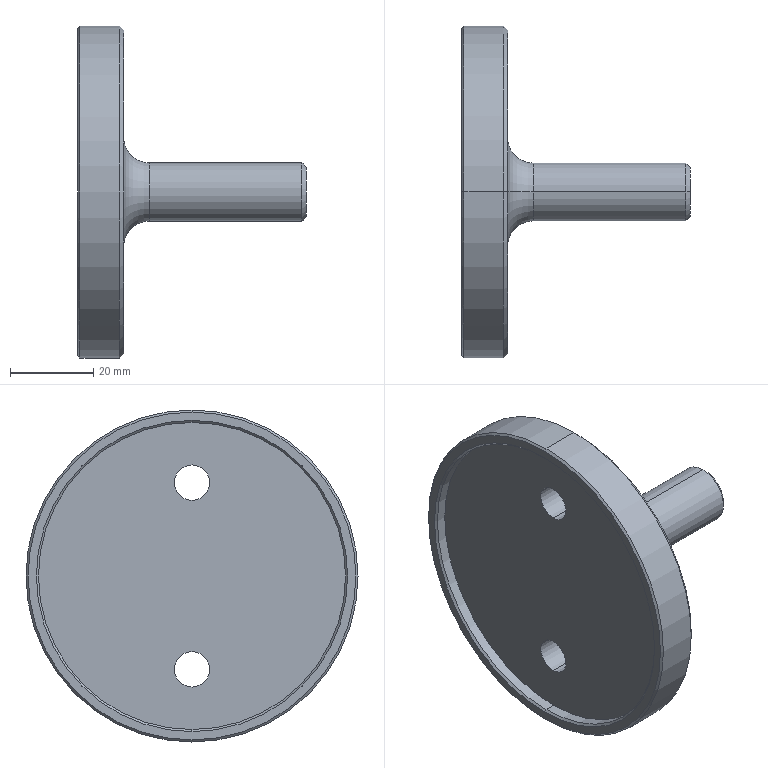Part | SolidWorks | features MBimport 1 | 1 solid | 24 faces | box 55 x 80 x 80 mm | volume 48487 mm3 | cylinder 10 | cone 8 | plane 4 | torus 2 | commonest cylinder face diameters 8.5 x4 14 x2 74 x2 80 x2
STEP:
#1=CARTESIAN_POINT('',(-14.582,0.,26.75));
#2=VERTEX_POINT('',#1);
#3=CARTESIAN_POINT('',(-6.582,0.,26.75));
#4=VERTEX_POINT('',#3);
#5=CARTESIAN_POINT('',(-16.582,0.,26.75));
#6=DIRECTION('',(1.,0.,0.));
#7=VECTOR('',#6,1000.);
#8=LINE('',#5,#7);
#9=EDGE_CURVE('',#2,#4,#8,.T.);
#10=ORIENTED_EDGE('',*,*,#9,.F.);
#11=CARTESIAN_POINT('',(-14.582,0.,18.25));
#12=VERTEX_POINT('',#11);
#13=CARTESIAN_POINT('',(-14.582,0.,22.5));
#14=DIRECTION('',(1.,0.,0.));
#15=DIRECTION('',(0.,0.,-1.));
#16=AXIS2_PLACEMENT_3D('',#13,#14,#15);
#17=CIRCLE('',#16,4.25);
#18=EDGE_CURVE('',#12,#2,#17,.T.);
#19=ORIENTED_EDGE('',*,*,#18,.F.);
#20=CARTESIAN_POINT('',(-6.582,0.,18.25));
#21=VERTEX_POINT('',#20);
#22=CARTESIAN_POINT('',(-16.582,0.,18.25));
#23=DIRECTION('',(1.,0.,0.));
#24=VECTOR('',#23,1000.);
#25=LINE('',#22,#24);
#26=EDGE_CURVE('',#12,#21,#25,.T.);
#27=ORIENTED_EDGE('',*,*,#26,.T.);
#28=CARTESIAN_POINT('',(-6.582,0.,22.5));
#29=DIRECTION('',(1.,0.,0.));
#30=DIRECTION('',(0.,0.,-1.));
#31=AXIS2_PLACEMENT_3D('',#28,#29,#30);
#32=CIRCLE('',#31,4.25);
#33=EDGE_CURVE('',#21,#4,#32,.T.);
#34=ORIENTED_EDGE('',*,*,#33,.T.);
#35=EDGE_LOOP('',(#10,#19,#27,#34));
#36=FACE_OUTER_BOUND('',#35,.T.);
#37=CARTESIAN_POINT('',(-16.582,0.,22.5));
#38=DIRECTION('',(1.,0.,0.));
#39=DIRECTION('',(0.,0.,-1.));
#40=AXIS2_PLACEMENT_3D('',#37,#38,#39);
#41=CYLINDRICAL_SURFACE('',#40,4.25);
#42=ADVANCED_FACE('',(#36),#41,.F.);
#43=CARTESIAN_POINT('',(-14.582,0.,-18.25));
#44=VERTEX_POINT('',#43);
#45=CARTESIAN_POINT('',(-6.582,0.,-18.25));
#46=VERTEX_POINT('',#45);
#47=CARTESIAN_POINT('',(-16.582,0.,-18.25));
#48=DIRECTION('',(1.,0.,0.));
#49=VECTOR('',#48,1000.);
#50=LINE('',#47,#49);
#51=EDGE_CURVE('',#44,#46,#50,.T.);
#52=ORIENTED_EDGE('',*,*,#51,.F.);
#53=CARTESIAN_POINT('',(-14.582,0.,-26.75));
#54=VERTEX_POINT('',#53);
#55=CARTESIAN_POINT('',(-14.582,0.,-22.5));
#56=DIRECTION('',(1.,0.,0.));
#57=DIRECTION('',(0.,0.,-1.));
#58=AXIS2_PLACEMENT_3D('',#55,#56,#57);
#59=CIRCLE('',#58,4.25);
#60=EDGE_CURVE('',#54,#44,#59,.T.);
#61=ORIENTED_EDGE('',*,*,#60,.F.);
#62=CARTESIAN_POINT('',(-6.582,0.,-26.75));
#63=VERTEX_POINT('',#62);
#64=CARTESIAN_POINT('',(-16.582,0.,-26.75));
#65=DIRECTION('',(1.,0.,0.));
#66=VECTOR('',#65,1000.);
#67=LINE('',#64,#66);
#68=EDGE_CURVE('',#54,#63,#67,.T.);
#69=ORIENTED_EDGE('',*,*,#68,.T.);
#70=CARTESIAN_POINT('',(-6.582,0.,-22.5));
#71=DIRECTION('',(1.,0.,0.));
#72=DIRECTION('',(0.,0.,-1.));
#73=AXIS2_PLACEMENT_3D('',#70,#71,#72);
#74=CIRCLE('',#73,4.25);
#75=EDGE_CURVE('',#63,#46,#74,.T.);
#76=ORIENTED_EDGE('',*,*,#75,.T.);
#77=EDGE_LOOP('',(#52,#61,#69,#76));
#78=FACE_OUTER_BOUND('',#77,.T.);
#79=CARTESIAN_POINT('',(-16.582,0.,-22.5));
#80=DIRECTION('',(1.,0.,0.));
#81=DIRECTION('',(0.,0.,-1.));
#82=AXIS2_PLACEMENT_3D('',#79,#80,#81);
#83=CYLINDRICAL_SURFACE('',#82,4.25);
#84=ADVANCED_FACE('',(#78),#83,.F.);
#85=CARTESIAN_POINT('',(37.418,0.,-6.));
#86=VERTEX_POINT('',#85);
#87=CARTESIAN_POINT('',(36.418,0.,-7.));
#88=VERTEX_POINT('',#87);
#89=CARTESIAN_POINT('',(36.418,0.,-7.));
#90=DIRECTION('',(-0.7071,0.,-0.7071));
#91=VECTOR('',#90,1000.);
#92=LINE('',#89,#91);
#93=EDGE_CURVE('',#86,#88,#92,.T.);
#94=ORIENTED_EDGE('',*,*,#93,.F.);
#95=CARTESIAN_POINT('',(37.418,0.,6.));
#96=VERTEX_POINT('',#95);
#97=CARTESIAN_POINT('',(37.418,0.,0.));
#98=DIRECTION('',(-1.,0.,0.));
#99=DIRECTION('',(0.,0.,1.));
#100=AXIS2_PLACEMENT_3D('',#97,#98,#99);
#101=CIRCLE('',#100,6.);
#102=EDGE_CURVE('',#86,#96,#101,.T.);
#103=ORIENTED_EDGE('',*,*,#102,.T.);
#104=CARTESIAN_POINT('',(36.418,0.,7.));
#105=VERTEX_POINT('',#104);
#106=CARTESIAN_POINT('',(36.418,0.,7.));
#107=DIRECTION('',(-0.7071,0.,0.7071));
#108=VECTOR('',#107,1000.);
#109=LINE('',#106,#108);
#110=EDGE_CURVE('',#96,#105,#109,.T.);
#111=ORIENTED_EDGE('',*,*,#110,.T.);
#112=CARTESIAN_POINT('',(36.418,0.,0.));
#113=DIRECTION('',(-1.,0.,0.));
#114=DIRECTION('',(0.,0.,1.));
#115=AXIS2_PLACEMENT_3D('',#112,#113,#114);
#116=CIRCLE('',#115,7.);
#117=EDGE_CURVE('',#88,#105,#116,.T.);
#118=ORIENTED_EDGE('',*,*,#117,.F.);
#119=EDGE_LOOP('',(#94,#103,#111,#118));
#120=FACE_OUTER_BOUND('',#119,.T.);
#121=CARTESIAN_POINT('',(36.418,0.,0.));
#122=DIRECTION('',(-1.,0.,0.));
#123=DIRECTION('',(0.,0.,1.));
#124=AXIS2_PLACEMENT_3D('',#121,#122,#123);
#125=CONICAL_SURFACE('',#124,7.,0.7854);
#126=ADVANCED_FACE('',(#120),#125,.T.);
#127=CARTESIAN_POINT('',(37.418,0.,0.));
#128=DIRECTION('',(-1.,0.,0.));
#129=DIRECTION('',(0.,0.,1.));
#130=AXIS2_PLACEMENT_3D('',#127,#128,#129);
#131=CIRCLE('',#130,6.);
#132=EDGE_CURVE('',#96,#86,#131,.T.);
#133=ORIENTED_EDGE('',*,*,#132,.F.);
#134=ORIENTED_EDGE('',*,*,#102,.F.);
#135=EDGE_LOOP('',(#133,#134));
#136=FACE_OUTER_BOUND('',#135,.T.);
#137=CARTESIAN_POINT('',(37.418,0.,0.));
#138=DIRECTION('',(1.,0.,0.));
#139=DIRECTION('',(0.,1.,0.));
#140=AXIS2_PLACEMENT_3D('',#137,#138,#139);
#141=PLANE('',#140);
#142=ADVANCED_FACE('',(#136),#141,.T.);
#143=ORIENTED_EDGE('',*,*,#60,.T.);
#144=CARTESIAN_POINT('',(-14.582,0.,-22.5));
#145=DIRECTION('',(1.,0.,0.));
#146=DIRECTION('',(0.,0.,-1.));
#147=AXIS2_PLACEMENT_3D('',#144,#145,#146);
#148=CIRCLE('',#147,4.25);
#149=EDGE_CURVE('',#44,#54,#148,.T.);
#150=ORIENTED_EDGE('',*,*,#149,.T.);
#151=EDGE_LOOP('',(#143,#150));
#152=FACE_BOUND('',#151,.T.);
#153=ORIENTED_EDGE('',*,*,#18,.T.);
#154=CARTESIAN_POINT('',(-14.582,0.,22.5));
#155=DIRECTION('',(1.,0.,0.));
#156=DIRECTION('',(0.,0.,-1.));
#157=AXIS2_PLACEMENT_3D('',#154,#155,#156);
#158=CIRCLE('',#157,4.25);
#159=EDGE_CURVE('',#2,#12,#158,.T.);
#160=ORIENTED_EDGE('',*,*,#159,.T.);
#161=EDGE_LOOP('',(#153,#160));
#162=FACE_BOUND('',#161,.T.);
#163=CARTESIAN_POINT('',(-14.582,0.,37.));
#164=VERTEX_POINT('',#163);
#165=CARTESIAN_POINT('',(-14.582,0.,-37.));
#166=VERTEX_POINT('',#165);
#167=CARTESIAN_POINT('',(-14.582,0.,0.));
#168=DIRECTION('',(-1.,0.,0.));
#169=DIRECTION('',(0.,0.,1.));
#170=AXIS2_PLACEMENT_3D('',#167,#168,#169);
#171=CIRCLE('',#170,37.);
#172=EDGE_CURVE('',#164,#166,#171,.T.);
#173=ORIENTED_EDGE('',*,*,#172,.T.);
#174=CARTESIAN_POINT('',(-14.582,0.,0.));
#175=DIRECTION('',(-1.,0.,0.));
#176=DIRECTION('',(0.,0.,1.));
#177=AXIS2_PLACEMENT_3D('',#174,#175,#176);
#178=CIRCLE('',#177,37.);
#179=EDGE_CURVE('',#166,#164,#178,.T.);
#180=ORIENTED_EDGE('',*,*,#179,.T.);
#181=EDGE_LOOP('',(#173,#180));
#182=FACE_OUTER_BOUND('',#181,.T.);
#183=CARTESIAN_POINT('',(-14.582,0.,0.));
#184=DIRECTION('',(1.,0.,0.));
#185=DIRECTION('',(0.,1.,0.));
#186=AXIS2_PLACEMENT_3D('',#183,#184,#185);
#187=PLANE('',#186);
#188=ADVANCED_FACE('',(#152,#162,#182),#187,.F.);
#189=CARTESIAN_POINT('',(-17.082,0.,-37.));
#190=VERTEX_POINT('',#189);
#191=CARTESIAN_POINT('',(-43.073,0.,-37.));
#192=DIRECTION('',(-1.,0.,0.));
#193=VECTOR('',#192,1000.);
#194=LINE('',#191,#193);
#195=EDGE_CURVE('',#166,#190,#194,.T.);
#196=ORIENTED_EDGE('',*,*,#195,.F.);
#197=ORIENTED_EDGE('',*,*,#172,.F.);
#198=CARTESIAN_POINT('',(-17.082,0.,37.));
#199=VERTEX_POINT('',#198);
#200=CARTESIAN_POINT('',(-43.073,0.,37.));
#201=DIRECTION('',(-1.,0.,0.));
#202=VECTOR('',#201,1000.);
#203=LINE('',#200,#202);
#204=EDGE_CURVE('',#164,#199,#203,.T.);
#205=ORIENTED_EDGE('',*,*,#204,.T.);
#206=CARTESIAN_POINT('',(-17.082,0.,0.));
#207=DIRECTION('',(-1.,0.,0.));
#208=DIRECTION('',(0.,0.,1.));
#209=AXIS2_PLACEMENT_3D('',#206,#207,#208);
#210=CIRCLE('',#209,37.);
#211=EDGE_CURVE('',#199,#190,#210,.T.);
#212=ORIENTED_EDGE('',*,*,#211,.T.);
#213=EDGE_LOOP('',(#196,#197,#205,#212));
#214=FACE_OUTER_BOUND('',#213,.T.);
#215=CARTESIAN_POINT('',(-43.073,0.,0.));
#216=DIRECTION('',(-1.,0.,0.));
#217=DIRECTION('',(0.,0.,1.));
#218=AXIS2_PLACEMENT_3D('',#215,#216,#217);
#219=CYLINDRICAL_SURFACE('',#218,37.);
#220=ADVANCED_FACE('',(#214),#219,.F.);
#221=CARTESIAN_POINT('',(-17.582,0.,-37.5));
#222=VERTEX_POINT('',#221);
#223=CARTESIAN_POINT('',(-17.582,0.,-37.5));
#224=DIRECTION('',(-0.7071,0.,-0.7071));
#225=VECTOR('',#224,1000.);
#226=LINE('',#223,#225);
#227=EDGE_CURVE('',#190,#222,#226,.T.);
#228=ORIENTED_EDGE('',*,*,#227,.F.);
#229=ORIENTED_EDGE('',*,*,#211,.F.);
#230=CARTESIAN_POINT('',(-17.582,0.,37.5));
#231=VERTEX_POINT('',#230);
#232=CARTESIAN_POINT('',(-17.582,0.,37.5));
#233=DIRECTION('',(-0.7071,0.,0.7071));
#234=VECTOR('',#233,1000.);
#235=LINE('',#232,#234);
#236=EDGE_CURVE('',#199,#231,#235,.T.);
#237=ORIENTED_EDGE('',*,*,#236,.T.);
#238=CARTESIAN_POINT('',(-17.582,0.,0.));
#239=DIRECTION('',(-1.,0.,0.));
#240=DIRECTION('',(0.,0.,1.));
#241=AXIS2_PLACEMENT_3D('',#238,#239,#240);
#242=CIRCLE('',#241,37.5);
#243=EDGE_CURVE('',#231,#222,#242,.T.);
#244=ORIENTED_EDGE('',*,*,#243,.T.);
#245=EDGE_LOOP('',(#228,#229,#237,#244));
#246=FACE_OUTER_BOUND('',#245,.T.);
#247=CARTESIAN_POINT('',(-17.582,0.,0.));
#248=DIRECTION('',(-1.,0.,0.));
#249=DIRECTION('',(0.,0.,1.));
#250=AXIS2_PLACEMENT_3D('',#247,#248,#249);
#251=CONICAL_SURFACE('',#250,37.5,0.7854);
#252=ADVANCED_FACE('',(#246),#251,.F.);
#253=ORIENTED_EDGE('',*,*,#243,.F.);
#254=CARTESIAN_POINT('',(-17.582,0.,0.));
#255=DIRECTION('',(-1.,0.,0.));
#256=DIRECTION('',(0.,0.,1.));
#257=AXIS2_PLACEMENT_3D('',#254,#255,#256);
#258=CIRCLE('',#257,37.5);
#259=EDGE_CURVE('',#222,#231,#258,.T.);
#260=ORIENTED_EDGE('',*,*,#259,.F.);
#261=EDGE_LOOP('',(#253,#260));
#262=FACE_BOUND('',#261,.T.);
#263=CARTESIAN_POINT('',(-17.582,0.,-39.5));
#264=VERTEX_POINT('',#263);
#265=CARTESIAN_POINT('',(-17.582,0.,39.5));
#266=VERTEX_POINT('',#265);
#267=CARTESIAN_POINT('',(-17.582,0.,0.));
#268=DIRECTION('',(-1.,0.,0.));
#269=DIRECTION('',(0.,0.,1.));
#270=AXIS2_PLACEMENT_3D('',#267,#268,#269);
#271=CIRCLE('',#270,39.5);
#272=EDGE_CURVE('',#264,#266,#271,.T.);
#273=ORIENTED_EDGE('',*,*,#272,.T.);
#274=CARTESIAN_POINT('',(-17.582,0.,0.));
#275=DIRECTION('',(-1.,0.,0.));
#276=DIRECTION('',(0.,0.,1.));
#277=AXIS2_PLACEMENT_3D('',#274,#275,#276);
#278=CIRCLE('',#277,39.5);
#279=EDGE_CURVE('',#266,#264,#278,.T.);
#280=ORIENTED_EDGE('',*,*,#279,.T.);
#281=EDGE_LOOP('',(#273,#280));
#282=FACE_OUTER_BOUND('',#281,.T.);
#283=CARTESIAN_POINT('',(-17.582,0.,0.));
#284=DIRECTION('',(-1.,0.,0.));
#285=DIRECTION('',(0.,0.,1.));
#286=AXIS2_PLACEMENT_3D('',#283,#284,#285);
#287=PLANE('',#286);
#288=ADVANCED_FACE('',(#262,#282),#287,.T.);
#289=CARTESIAN_POINT('',(-17.082,0.,40.));
#290=VERTEX_POINT('',#289);
#291=CARTESIAN_POINT('',(-17.582,0.,39.5));
#292=DIRECTION('',(0.7071,0.,0.7071));
#293=VECTOR('',#292,1000.);
#294=LINE('',#291,#293);
#295=EDGE_CURVE('',#266,#290,#294,.T.);
#296=ORIENTED_EDGE('',*,*,#295,.F.);
#297=ORIENTED_EDGE('',*,*,#272,.F.);
#298=CARTESIAN_POINT('',(-17.082,0.,-40.));
#299=VERTEX_POINT('',#298);
#300=CARTESIAN_POINT('',(-17.582,0.,-39.5));
#301=DIRECTION('',(0.7071,0.,-0.7071));
#302=VECTOR('',#301,1000.);
#303=LINE('',#300,#302);
#304=EDGE_CURVE('',#264,#299,#303,.T.);
#305=ORIENTED_EDGE('',*,*,#304,.T.);
#306=CARTESIAN_POINT('',(-17.082,0.,0.));
#307=DIRECTION('',(-1.,0.,0.));
#308=DIRECTION('',(0.,0.,1.));
#309=AXIS2_PLACEMENT_3D('',#306,#307,#308);
#310=CIRCLE('',#309,40.);
#311=EDGE_CURVE('',#299,#290,#310,.T.);
#312=ORIENTED_EDGE('',*,*,#311,.T.);
#313=EDGE_LOOP('',(#296,#297,#305,#312));
#314=FACE_OUTER_BOUND('',#313,.T.);
#315=CARTESIAN_POINT('',(-17.582,0.,0.));
#316=DIRECTION('',(1.,0.,0.));
#317=DIRECTION('',(0.,0.,-1.));
#318=AXIS2_PLACEMENT_3D('',#315,#316,#317);
#319=CONICAL_SURFACE('',#318,39.5,0.7854);
#320=ADVANCED_FACE('',(#314),#319,.T.);
#321=CARTESIAN_POINT('',(-7.582,0.,-40.));
#322=VERTEX_POINT('',#321);
#323=CARTESIAN_POINT('',(-43.073,0.,-40.));
#324=DIRECTION('',(-1.,0.,0.));
#325=VECTOR('',#324,1000.);
#326=LINE('',#323,#325);
#327=EDGE_CURVE('',#322,#299,#326,.T.);
#328=ORIENTED_EDGE('',*,*,#327,.F.);
#329=CARTESIAN_POINT('',(-7.582,0.,40.));
#330=VERTEX_POINT('',#329);
#331=CARTESIAN_POINT('',(-7.582,0.,0.));
#332=DIRECTION('',(-1.,0.,0.));
#333=DIRECTION('',(0.,0.,1.));
#334=AXIS2_PLACEMENT_3D('',#331,#332,#333);
#335=CIRCLE('',#334,40.);
#336=EDGE_CURVE('',#322,#330,#335,.T.);
#337=ORIENTED_EDGE('',*,*,#336,.T.);
#338=CARTESIAN_POINT('',(-43.073,0.,40.));
#339=DIRECTION('',(-1.,0.,0.));
#340=VECTOR('',#339,1000.);
#341=LINE('',#338,#340);
#342=EDGE_CURVE('',#330,#290,#341,.T.);
#343=ORIENTED_EDGE('',*,*,#342,.T.);
#344=ORIENTED_EDGE('',*,*,#311,.F.);
#345=EDGE_LOOP('',(#328,#337,#343,#344));
#346=FACE_OUTER_BOUND('',#345,.T.);
#347=CARTESIAN_POINT('',(-43.073,0.,0.));
#348=DIRECTION('',(-1.,0.,0.));
#349=DIRECTION('',(0.,0.,1.));
#350=AXIS2_PLACEMENT_3D('',#347,#348,#349);
#351=CYLINDRICAL_SURFACE('',#350,40.);
#352=ADVANCED_FACE('',(#346),#351,.T.);
#353=CARTESIAN_POINT('',(-6.582,0.,-39.));
#354=VERTEX_POINT('',#353);
#355=CARTESIAN_POINT('',(-7.582,0.,-40.));
#356=DIRECTION('',(-0.7071,0.,-0.7071));
#357=VECTOR('',#356,1000.);
#358=LINE('',#355,#357);
#359=EDGE_CURVE('',#354,#322,#358,.T.);
#360=ORIENTED_EDGE('',*,*,#359,.F.);
#361=CARTESIAN_POINT('',(-6.582,0.,39.));
#362=VERTEX_POINT('',#361);
#363=CARTESIAN_POINT('',(-6.582,0.,0.));
#364=DIRECTION('',(-1.,0.,0.));
#365=DIRECTION('',(0.,0.,1.));
#366=AXIS2_PLACEMENT_3D('',#363,#364,#365);
#367=CIRCLE('',#366,39.);
#368=EDGE_CURVE('',#354,#362,#367,.T.);
#369=ORIENTED_EDGE('',*,*,#368,.T.);
#370=CARTESIAN_POINT('',(-7.582,0.,40.));
#371=DIRECTION('',(-0.7071,0.,0.7071));
#372=VECTOR('',#371,1000.);
#373=LINE('',#370,#372);
#374=EDGE_CURVE('',#362,#330,#373,.T.);
#375=ORIENTED_EDGE('',*,*,#374,.T.);
#376=ORIENTED_EDGE('',*,*,#336,.F.);
#377=EDGE_LOOP('',(#360,#369,#375,#376));
#378=FACE_OUTER_BOUND('',#377,.T.);
#379=CARTESIAN_POINT('',(-7.582,0.,0.));
#380=DIRECTION('',(-1.,0.,0.));
#381=DIRECTION('',(0.,0.,1.));
#382=AXIS2_PLACEMENT_3D('',#379,#380,#381);
#383=CONICAL_SURFACE('',#382,40.,0.7854);
#384=ADVANCED_FACE('',(#378),#383,.T.);
#385=CARTESIAN_POINT('',(-6.582,0.,13.226));
#386=VERTEX_POINT('',#385);
#387=CARTESIAN_POINT('',(-6.582,0.,-13.226));
#388=VERTEX_POINT('',#387);
#389=CARTESIAN_POINT('',(-6.582,0.,0.));
#390=DIRECTION('',(-1.,0.,0.));
#391=DIRECTION('',(0.,0.,1.));
#392=AXIS2_PLACEMENT_3D('',#389,#390,#391);
#393=CIRCLE('',#392,13.226);
#394=EDGE_CURVE('',#386,#388,#393,.T.);
#395=ORIENTED_EDGE('',*,*,#394,.T.);
#396=CARTESIAN_POINT('',(-6.582,0.,0.));
#397=DIRECTION('',(-1.,0.,0.));
#398=DIRECTION('',(0.,0.,1.));
#399=AXIS2_PLACEMENT_3D('',#396,#397,#398);
#400=CIRCLE('',#399,13.226);
#401=EDGE_CURVE('',#388,#386,#400,.T.);
#402=ORIENTED_EDGE('',*,*,#401,.T.);
#403=EDGE_LOOP('',(#395,#402));
#404=FACE_BOUND('',#403,.T.);
#405=ORIENTED_EDGE('',*,*,#75,.F.);
#406=CARTESIAN_POINT('',(-6.582,0.,-22.5));
#407=DIRECTION('',(1.,0.,0.));
#408=DIRECTION('',(0.,0.,-1.));
#409=AXIS2_PLACEMENT_3D('',#406,#407,#408);
#410=CIRCLE('',#409,4.25);
#411=EDGE_CURVE('',#46,#63,#410,.T.);
#412=ORIENTED_EDGE('',*,*,#411,.F.);
#413=EDGE_LOOP('',(#405,#412));
#414=FACE_BOUND('',#413,.T.);
#415=ORIENTED_EDGE('',*,*,#33,.F.);
#416=CARTESIAN_POINT('',(-6.582,0.,22.5));
#417=DIRECTION('',(1.,0.,0.));
#418=DIRECTION('',(0.,0.,-1.));
#419=AXIS2_PLACEMENT_3D('',#416,#417,#418);
#420=CIRCLE('',#419,4.25);
#421=EDGE_CURVE('',#4,#21,#420,.T.);
#422=ORIENTED_EDGE('',*,*,#421,.F.);
#423=EDGE_LOOP('',(#415,#422));
#424=FACE_BOUND('',#423,.T.);
#425=CARTESIAN_POINT('',(-6.582,0.,0.));
#426=DIRECTION('',(-1.,0.,0.));
#427=DIRECTION('',(0.,0.,1.));
#428=AXIS2_PLACEMENT_3D('',#425,#426,#427);
#429=CIRCLE('',#428,39.);
#430=EDGE_CURVE('',#362,#354,#429,.T.);
#431=ORIENTED_EDGE('',*,*,#430,.F.);
#432=ORIENTED_EDGE('',*,*,#368,.F.);
#433=EDGE_LOOP('',(#431,#432));
#434=FACE_OUTER_BOUND('',#433,.T.);
#435=CARTESIAN_POINT('',(-6.582,0.,0.));
#436=DIRECTION('',(1.,0.,0.));
#437=DIRECTION('',(0.,1.,0.));
#438=AXIS2_PLACEMENT_3D('',#435,#436,#437);
#439=PLANE('',#438);
#440=ADVANCED_FACE('',(#404,#414,#424,#434),#439,.T.);
#441=CARTESIAN_POINT('',(-0.3561,0.,-7.));
#442=VERTEX_POINT('',#441);
#443=CARTESIAN_POINT('',(-0.3561,0.,-13.226));
#444=DIRECTION('',(0.,1.,0.));
#445=DIRECTION('',(0.,0.,1.));
#446=AXIS2_PLACEMENT_3D('',#443,#444,#445);
#447=CIRCLE('',#446,6.226);
#448=EDGE_CURVE('',#388,#442,#447,.T.);
#449=ORIENTED_EDGE('',*,*,#448,.F.);
#450=ORIENTED_EDGE('',*,*,#394,.F.);
#451=CARTESIAN_POINT('',(-0.3561,0.,7.));
#452=VERTEX_POINT('',#451);
#453=CARTESIAN_POINT('',(-0.3561,0.,13.226));
#454=DIRECTION('',(0.,-1.,0.));
#455=DIRECTION('',(0.,0.,-1.));
#456=AXIS2_PLACEMENT_3D('',#453,#454,#455);
#457=CIRCLE('',#456,6.226);
#458=EDGE_CURVE('',#386,#452,#457,.T.);
#459=ORIENTED_EDGE('',*,*,#458,.T.);
#460=CARTESIAN_POINT('',(-0.3561,0.,0.));
#461=DIRECTION('',(-1.,0.,0.));
#462=DIRECTION('',(0.,0.,1.));
#463=AXIS2_PLACEMENT_3D('',#460,#461,#462);
#464=CIRCLE('',#463,7.);
#465=EDGE_CURVE('',#452,#442,#464,.T.);
#466=ORIENTED_EDGE('',*,*,#465,.T.);
#467=EDGE_LOOP('',(#449,#450,#459,#466));
#468=FACE_OUTER_BOUND('',#467,.T.);
#469=CARTESIAN_POINT('',(-0.3561,0.,0.));
#470=DIRECTION('',(-1.,0.,0.));
#471=DIRECTION('',(0.,0.,1.));
#472=AXIS2_PLACEMENT_3D('',#469,#470,#471);
#473=TOROIDAL_SURFACE('',#472,13.226,6.226);
#474=ADVANCED_FACE('',(#468),#473,.F.);
#475=CARTESIAN_POINT('',(-43.073,0.,-7.));
#476=DIRECTION('',(-1.,0.,0.));
#477=VECTOR('',#476,1000.);
#478=LINE('',#475,#477);
#479=EDGE_CURVE('',#88,#442,#478,.T.);
#480=ORIENTED_EDGE('',*,*,#479,.F.);
#481=ORIENTED_EDGE('',*,*,#117,.T.);
#482=CARTESIAN_POINT('',(-43.073,0.,7.));
#483=DIRECTION('',(-1.,0.,0.));
#484=VECTOR('',#483,1000.);
#485=LINE('',#482,#484);
#486=EDGE_CURVE('',#105,#452,#485,.T.);
#487=ORIENTED_EDGE('',*,*,#486,.T.);
#488=CARTESIAN_POINT('',(-0.3561,0.,0.));
#489=DIRECTION('',(-1.,0.,0.));
#490=DIRECTION('',(0.,0.,1.));
#491=AXIS2_PLACEMENT_3D('',#488,#489,#490);
#492=CIRCLE('',#491,7.);
#493=EDGE_CURVE('',#442,#452,#492,.T.);
#494=ORIENTED_EDGE('',*,*,#493,.F.);
#495=EDGE_LOOP('',(#480,#481,#487,#494));
#496=FACE_OUTER_BOUND('',#495,.T.);
#497=CARTESIAN_POINT('',(-43.073,0.,0.));
#498=DIRECTION('',(-1.,0.,0.));
#499=DIRECTION('',(0.,0.,1.));
#500=AXIS2_PLACEMENT_3D('',#497,#498,#499);
#501=CYLINDRICAL_SURFACE('',#500,7.);
#502=ADVANCED_FACE('',(#496),#501,.T.);
#503=CARTESIAN_POINT('',(36.418,0.,0.));
#504=DIRECTION('',(-1.,0.,0.));
#505=DIRECTION('',(0.,0.,1.));
#506=AXIS2_PLACEMENT_3D('',#503,#504,#505);
#507=CIRCLE('',#506,7.);
#508=EDGE_CURVE('',#105,#88,#507,.T.);
#509=ORIENTED_EDGE('',*,*,#508,.T.);
#510=ORIENTED_EDGE('',*,*,#479,.T.);
#511=ORIENTED_EDGE('',*,*,#465,.F.);
#512=ORIENTED_EDGE('',*,*,#486,.F.);
#513=EDGE_LOOP('',(#509,#510,#511,#512));
#514=FACE_OUTER_BOUND('',#513,.T.);
#515=CARTESIAN_POINT('',(-43.073,0.,0.));
#516=DIRECTION('',(-1.,0.,0.));
#517=DIRECTION('',(0.,0.,1.));
#518=AXIS2_PLACEMENT_3D('',#515,#516,#517);
#519=CYLINDRICAL_SURFACE('',#518,7.);
#520=ADVANCED_FACE('',(#514),#519,.T.);
#521=ORIENTED_EDGE('',*,*,#401,.F.);
#522=ORIENTED_EDGE('',*,*,#448,.T.);
#523=ORIENTED_EDGE('',*,*,#493,.T.);
#524=ORIENTED_EDGE('',*,*,#458,.F.);
#525=EDGE_LOOP('',(#521,#522,#523,#524));
#526=FACE_OUTER_BOUND('',#525,.T.);
#527=CARTESIAN_POINT('',(-0.3561,0.,0.));
#528=DIRECTION('',(-1.,0.,0.));
#529=DIRECTION('',(0.,0.,1.));
#530=AXIS2_PLACEMENT_3D('',#527,#528,#529);
#531=TOROIDAL_SURFACE('',#530,13.226,6.226);
#532=ADVANCED_FACE('',(#526),#531,.F.);
#533=ORIENTED_EDGE('',*,*,#430,.T.);
#534=ORIENTED_EDGE('',*,*,#359,.T.);
#535=CARTESIAN_POINT('',(-7.582,0.,0.));
#536=DIRECTION('',(-1.,0.,0.));
#537=DIRECTION('',(0.,0.,1.));
#538=AXIS2_PLACEMENT_3D('',#535,#536,#537);
#539=CIRCLE('',#538,40.);
#540=EDGE_CURVE('',#330,#322,#539,.T.);
#541=ORIENTED_EDGE('',*,*,#540,.F.);
#542=ORIENTED_EDGE('',*,*,#374,.F.);
#543=EDGE_LOOP('',(#533,#534,#541,#542));
#544=FACE_OUTER_BOUND('',#543,.T.);
#545=CARTESIAN_POINT('',(-7.582,0.,0.));
#546=DIRECTION('',(-1.,0.,0.));
#547=DIRECTION('',(0.,0.,1.));
#548=AXIS2_PLACEMENT_3D('',#545,#546,#547);
#549=CONICAL_SURFACE('',#548,40.,0.7854);
#550=ADVANCED_FACE('',(#544),#549,.T.);
#551=ORIENTED_EDGE('',*,*,#540,.T.);
#552=ORIENTED_EDGE('',*,*,#327,.T.);
#553=CARTESIAN_POINT('',(-17.082,0.,0.));
#554=DIRECTION('',(-1.,0.,0.));
#555=DIRECTION('',(0.,0.,1.));
#556=AXIS2_PLACEMENT_3D('',#553,#554,#555);
#557=CIRCLE('',#556,40.);
#558=EDGE_CURVE('',#290,#299,#557,.T.);
#559=ORIENTED_EDGE('',*,*,#558,.F.);
#560=ORIENTED_EDGE('',*,*,#342,.F.);
#561=EDGE_LOOP('',(#551,#552,#559,#560));
#562=FACE_OUTER_BOUND('',#561,.T.);
#563=CARTESIAN_POINT('',(-43.073,0.,0.));
#564=DIRECTION('',(-1.,0.,0.));
#565=DIRECTION('',(0.,0.,1.));
#566=AXIS2_PLACEMENT_3D('',#563,#564,#565);
#567=CYLINDRICAL_SURFACE('',#566,40.);
#568=ADVANCED_FACE('',(#562),#567,.T.);
#569=ORIENTED_EDGE('',*,*,#279,.F.);
#570=ORIENTED_EDGE('',*,*,#295,.T.);
#571=ORIENTED_EDGE('',*,*,#558,.T.);
#572=ORIENTED_EDGE('',*,*,#304,.F.);
#573=EDGE_LOOP('',(#569,#570,#571,#572));
#574=FACE_OUTER_BOUND('',#573,.T.);
#575=CARTESIAN_POINT('',(-17.582,0.,0.));
#576=DIRECTION('',(1.,0.,0.));
#577=DIRECTION('',(0.,0.,-1.));
#578=AXIS2_PLACEMENT_3D('',#575,#576,#577);
#579=CONICAL_SURFACE('',#578,39.5,0.7854);
#580=ADVANCED_FACE('',(#574),#579,.T.);
#581=CARTESIAN_POINT('',(-17.082,0.,0.));
#582=DIRECTION('',(-1.,0.,0.));
#583=DIRECTION('',(0.,0.,1.));
#584=AXIS2_PLACEMENT_3D('',#581,#582,#583);
#585=CIRCLE('',#584,37.);
#586=EDGE_CURVE('',#190,#199,#585,.T.);
#587=ORIENTED_EDGE('',*,*,#586,.F.);
#588=ORIENTED_EDGE('',*,*,#227,.T.);
#589=ORIENTED_EDGE('',*,*,#259,.T.);
#590=ORIENTED_EDGE('',*,*,#236,.F.);
#591=EDGE_LOOP('',(#587,#588,#589,#590));
#592=FACE_OUTER_BOUND('',#591,.T.);
#593=CARTESIAN_POINT('',(-17.582,0.,0.));
#594=DIRECTION('',(-1.,0.,0.));
#595=DIRECTION('',(0.,0.,1.));
#596=AXIS2_PLACEMENT_3D('',#593,#594,#595);
#597=CONICAL_SURFACE('',#596,37.5,0.7854);
#598=ADVANCED_FACE('',(#592),#597,.F.);
#599=ORIENTED_EDGE('',*,*,#179,.F.);
#600=ORIENTED_EDGE('',*,*,#195,.T.);
#601=ORIENTED_EDGE('',*,*,#586,.T.);
#602=ORIENTED_EDGE('',*,*,#204,.F.);
#603=EDGE_LOOP('',(#599,#600,#601,#602));
#604=FACE_OUTER_BOUND('',#603,.T.);
#605=CARTESIAN_POINT('',(-43.073,0.,0.));
#606=DIRECTION('',(-1.,0.,0.));
#607=DIRECTION('',(0.,0.,1.));
#608=AXIS2_PLACEMENT_3D('',#605,#606,#607);
#609=CYLINDRICAL_SURFACE('',#608,37.);
#610=ADVANCED_FACE('',(#604),#609,.F.);
#611=ORIENTED_EDGE('',*,*,#132,.T.);
#612=ORIENTED_EDGE('',*,*,#93,.T.);
#613=ORIENTED_EDGE('',*,*,#508,.F.);
#614=ORIENTED_EDGE('',*,*,#110,.F.);
#615=EDGE_LOOP('',(#611,#612,#613,#614));
#616=FACE_OUTER_BOUND('',#615,.T.);
#617=CARTESIAN_POINT('',(36.418,0.,0.));
#618=DIRECTION('',(-1.,0.,0.));
#619=DIRECTION('',(0.,0.,1.));
#620=AXIS2_PLACEMENT_3D('',#617,#618,#619);
#621=CONICAL_SURFACE('',#620,7.,0.7854);
#622=ADVANCED_FACE('',(#616),#621,.T.);
#623=ORIENTED_EDGE('',*,*,#149,.F.);
#624=ORIENTED_EDGE('',*,*,#51,.T.);
#625=ORIENTED_EDGE('',*,*,#411,.T.);
#626=ORIENTED_EDGE('',*,*,#68,.F.);
#627=EDGE_LOOP('',(#623,#624,#625,#626));
#628=FACE_OUTER_BOUND('',#627,.T.);
#629=CARTESIAN_POINT('',(-16.582,0.,-22.5));
#630=DIRECTION('',(1.,0.,0.));
#631=DIRECTION('',(0.,0.,-1.));
#632=AXIS2_PLACEMENT_3D('',#629,#630,#631);
#633=CYLINDRICAL_SURFACE('',#632,4.25);
#634=ADVANCED_FACE('',(#628),#633,.F.);
#635=ORIENTED_EDGE('',*,*,#159,.F.);
#636=ORIENTED_EDGE('',*,*,#9,.T.);
#637=ORIENTED_EDGE('',*,*,#421,.T.);
#638=ORIENTED_EDGE('',*,*,#26,.F.);
#639=EDGE_LOOP('',(#635,#636,#637,#638));
#640=FACE_OUTER_BOUND('',#639,.T.);
#641=CARTESIAN_POINT('',(-16.582,0.,22.5));
#642=DIRECTION('',(1.,0.,0.));
#643=DIRECTION('',(0.,0.,-1.));
#644=AXIS2_PLACEMENT_3D('',#641,#642,#643);
#645=CYLINDRICAL_SURFACE('',#644,4.25);
#646=ADVANCED_FACE('',(#640),#645,.F.);
#647=CLOSED_SHELL('',(#42,#84,#126,#142,#188,#220,#252,#288,#320,#352,#384,#440,#474,#502,#520,#532,#550,#568,#580,#598,#610,#622,#634,#646));
#648=MANIFOLD_SOLID_BREP('',#647);
#649=CARTESIAN_POINT('',(0.,0.,0.));
#650=DIRECTION('',(0.,0.,1.));
#651=DIRECTION('',(1.,0.,0.));
#652=AXIS2_PLACEMENT_3D('',#649,#650,#651);
#653=(LENGTH_UNIT()NAMED_UNIT(*)SI_UNIT(.MILLI.,.METRE.));
#654=UNCERTAINTY_MEASURE_WITH_UNIT(LENGTH_MEASURE(0.00001),#653,'','');
#655=(NAMED_UNIT(*)PLANE_ANGLE_UNIT()SI_UNIT($,.RADIAN.));
#656=(NAMED_UNIT(*)SI_UNIT($,.STERADIAN.)SOLID_ANGLE_UNIT());
#657=(GEOMETRIC_REPRESENTATION_CONTEXT(3)GLOBAL_UNCERTAINTY_ASSIGNED_CONTEXT((#654))GLOBAL_UNIT_ASSIGNED_CONTEXT((#653,#655,#656))REPRESENTATION_CONTEXT('',''));
#658=ADVANCED_BREP_SHAPE_REPRESENTATION('',(#648,#652),#657);